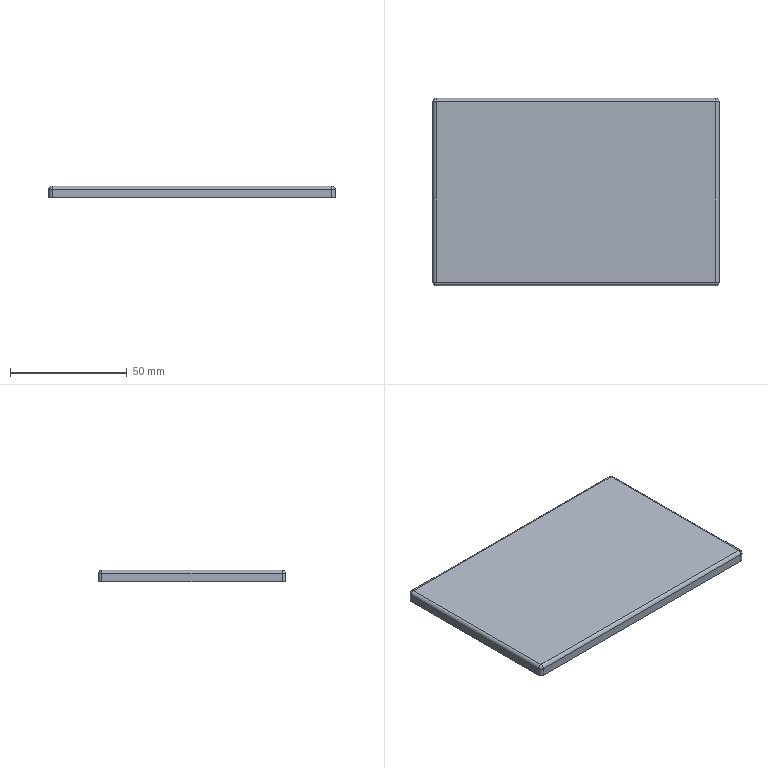Part | STEP file | ASND-0110-SDS_4 | 1 solid | 23 faces | box 122.6 x 80.2 x 5 mm | volume 16643 mm3 | plane 11 | cylinder 8 | sphere 4 | commonest cylinder face diameters 3 x8